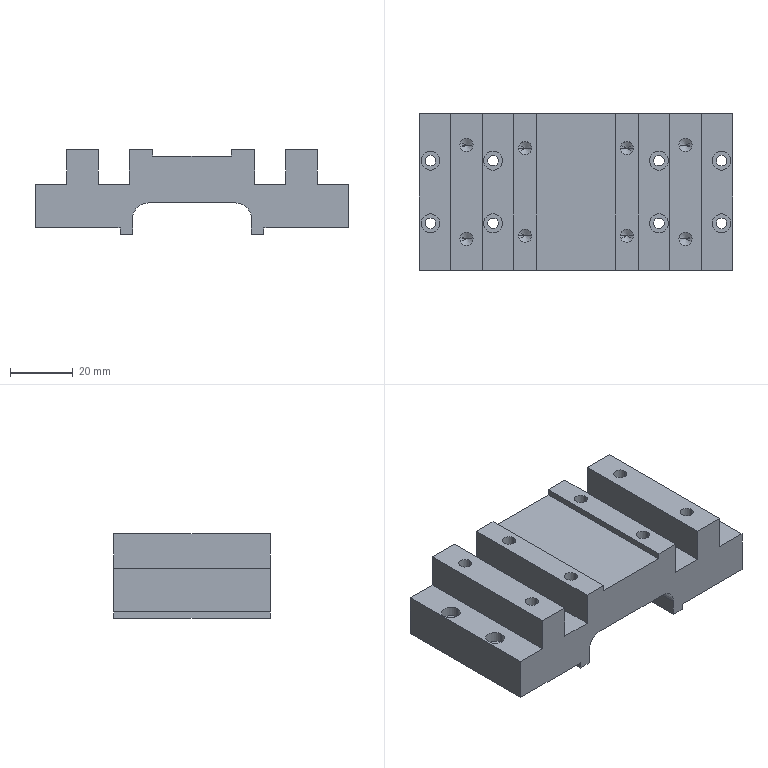Part | 1 solid | 104 faces | box 100 x 50 x 27 mm | volume 83499 mm3 | cylinder 50 | plane 38 | cone 16 | commonest cylinder face diameters 3.4 x16 4.2 x16 6 x16 10 x2